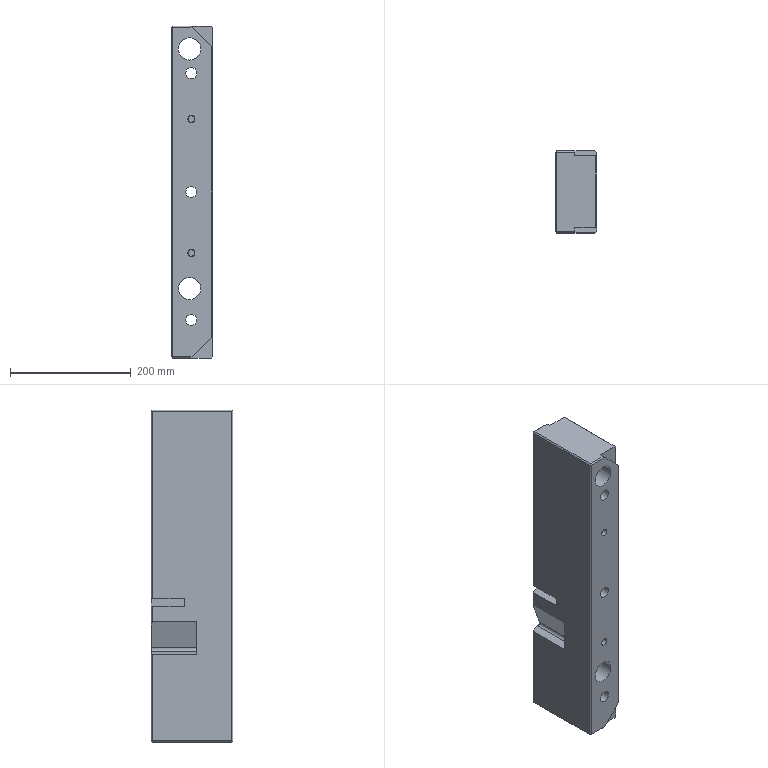Part | STEP file | SPACE-PLATE_id502_x_t | 1 solid | 48 faces | box 68 x 135 x 550 mm | volume 4551876 mm3 | plane 37 | cylinder 9 | cone 2 | commonest cylinder face diameters 18.5 x3 10 x2 12 x2 37 x2
STEP:
#1=CARTESIAN_POINT('',(165.,-234.5,115.75));
#2=VERTEX_POINT('',#1);
#3=CARTESIAN_POINT('',(165.,-234.5,121.));
#4=DIRECTION('',(0.,-1.,0.));
#5=DIRECTION('',(0.,0.,-1.));
#6=AXIS2_PLACEMENT_3D('',#3,#4,#5);
#7=CIRCLE('',#6,5.25);
#8=EDGE_CURVE('',#2,#2,#7,.T.);
#9=ORIENTED_EDGE('',*,*,#8,.T.);
#10=EDGE_LOOP('',(#9));
#11=FACE_OUTER_BOUND('',#10,.T.);
#12=CARTESIAN_POINT('',(165.,-234.5,121.));
#13=DIRECTION('',(0.,1.,0.));
#14=DIRECTION('',(0.,0.,1.));
#15=AXIS2_PLACEMENT_3D('',#12,#13,#14);
#16=PLANE('',#15);
#17=ADVANCED_FACE('',(#11),#16,.F.);
#18=CARTESIAN_POINT('',(165.,-234.5,-106.25));
#19=VERTEX_POINT('',#18);
#20=CARTESIAN_POINT('',(165.,-234.5,-101.));
#21=DIRECTION('',(0.,-1.,0.));
#22=DIRECTION('',(0.,0.,-1.));
#23=AXIS2_PLACEMENT_3D('',#20,#21,#22);
#24=CIRCLE('',#23,5.25);
#25=EDGE_CURVE('',#19,#19,#24,.T.);
#26=ORIENTED_EDGE('',*,*,#25,.T.);
#27=EDGE_LOOP('',(#26));
#28=FACE_OUTER_BOUND('',#27,.T.);
#29=CARTESIAN_POINT('',(165.,-234.5,-101.));
#30=DIRECTION('',(0.,-1.,0.));
#31=DIRECTION('',(0.,0.,-1.));
#32=AXIS2_PLACEMENT_3D('',#29,#30,#31);
#33=PLANE('',#32);
#34=ADVANCED_FACE('',(#28),#33,.T.);
#35=CARTESIAN_POINT('',(165.,-235.25,127.));
#36=VERTEX_POINT('',#35);
#37=CARTESIAN_POINT('',(165.,-235.25,121.));
#38=DIRECTION('',(0.,-1.,0.));
#39=DIRECTION('',(0.,0.,1.));
#40=AXIS2_PLACEMENT_3D('',#37,#38,#39);
#41=CIRCLE('',#40,6.);
#42=EDGE_CURVE('',#36,#36,#41,.T.);
#43=ORIENTED_EDGE('',*,*,#42,.T.);
#44=EDGE_LOOP('',(#43));
#45=FACE_BOUND('',#44,.T.);
#46=ORIENTED_EDGE('',*,*,#8,.F.);
#47=EDGE_LOOP('',(#46));
#48=FACE_BOUND('',#47,.T.);
#49=CARTESIAN_POINT('',(165.,-235.25,121.));
#50=DIRECTION('',(0.,-1.,0.));
#51=DIRECTION('',(0.,0.,-1.));
#52=AXIS2_PLACEMENT_3D('',#49,#50,#51);
#53=CONICAL_SURFACE('',#52,6.,45.);
#54=ADVANCED_FACE('',(#45,#48),#53,.F.);
#55=CARTESIAN_POINT('',(165.,-235.25,-107.));
#56=VERTEX_POINT('',#55);
#57=CARTESIAN_POINT('',(165.,-235.25,-101.));
#58=DIRECTION('',(0.,-1.,0.));
#59=DIRECTION('',(0.,0.,-1.));
#60=AXIS2_PLACEMENT_3D('',#57,#58,#59);
#61=CIRCLE('',#60,6.);
#62=EDGE_CURVE('',#56,#56,#61,.T.);
#63=ORIENTED_EDGE('',*,*,#62,.T.);
#64=EDGE_LOOP('',(#63));
#65=FACE_BOUND('',#64,.T.);
#66=ORIENTED_EDGE('',*,*,#25,.F.);
#67=EDGE_LOOP('',(#66));
#68=FACE_BOUND('',#67,.T.);
#69=CARTESIAN_POINT('',(165.,-235.25,-101.));
#70=DIRECTION('',(0.,-1.,0.));
#71=DIRECTION('',(0.,0.,-1.));
#72=AXIS2_PLACEMENT_3D('',#69,#70,#71);
#73=CONICAL_SURFACE('',#72,6.,45.);
#74=ADVANCED_FACE('',(#65,#68),#73,.F.);
#75=CARTESIAN_POINT('',(144.313,-195.5,-125.297));
#76=VERTEX_POINT('',#75);
#77=CARTESIAN_POINT('',(132.,-195.5,-129.657));
#78=VERTEX_POINT('',#77);
#79=CARTESIAN_POINT('',(144.313,-195.5,-125.297));
#80=DIRECTION('',(-0.9426,0.,-0.3338));
#81=VECTOR('',#80,1.);
#82=LINE('',#79,#81);
#83=EDGE_CURVE('',#76,#78,#82,.T.);
#84=ORIENTED_EDGE('',*,*,#83,.T.);
#85=CARTESIAN_POINT('',(132.,-195.5,-75.548));
#86=VERTEX_POINT('',#85);
#87=CARTESIAN_POINT('',(132.,-195.5,275.));
#88=DIRECTION('',(0.,0.,-1.));
#89=VECTOR('',#88,1.);
#90=LINE('',#87,#89);
#91=EDGE_CURVE('',#86,#78,#90,.T.);
#92=ORIENTED_EDGE('',*,*,#91,.F.);
#93=CARTESIAN_POINT('',(147.357,-195.5,-118.915));
#94=VERTEX_POINT('',#93);
#95=CARTESIAN_POINT('',(132.,-195.5,-75.548));
#96=DIRECTION('',(0.3338,0.,-0.9426));
#97=VECTOR('',#96,1.);
#98=LINE('',#95,#97);
#99=EDGE_CURVE('',#86,#94,#98,.T.);
#100=ORIENTED_EDGE('',*,*,#99,.T.);
#101=CARTESIAN_POINT('',(142.644,-195.5,-120.584));
#102=DIRECTION('',(0.,1.,0.));
#103=DIRECTION('',(0.,0.,1.));
#104=AXIS2_PLACEMENT_3D('',#101,#102,#103);
#105=CIRCLE('',#104,5.);
#106=EDGE_CURVE('',#94,#76,#105,.T.);
#107=ORIENTED_EDGE('',*,*,#106,.T.);
#108=EDGE_LOOP('',(#84,#92,#100,#107));
#109=FACE_OUTER_BOUND('',#108,.T.);
#110=CARTESIAN_POINT('',(-225.,-195.5,275.));
#111=DIRECTION('',(0.,1.,0.));
#112=DIRECTION('',(0.,0.,1.));
#113=AXIS2_PLACEMENT_3D('',#110,#111,#112);
#114=PLANE('',#113);
#115=ADVANCED_FACE('',(#109),#114,.T.);
#116=CARTESIAN_POINT('',(173.488,-175.5,-35.932));
#117=VERTEX_POINT('',#116);
#118=CARTESIAN_POINT('',(132.,-175.5,-50.624));
#119=VERTEX_POINT('',#118);
#120=CARTESIAN_POINT('',(173.488,-175.5,-35.932));
#121=DIRECTION('',(-0.9426,0.,-0.3338));
#122=VECTOR('',#121,1.);
#123=LINE('',#120,#122);
#124=EDGE_CURVE('',#117,#119,#123,.T.);
#125=ORIENTED_EDGE('',*,*,#124,.T.);
#126=CARTESIAN_POINT('',(132.,-175.5,-36.833));
#127=VERTEX_POINT('',#126);
#128=CARTESIAN_POINT('',(132.,-175.5,275.));
#129=DIRECTION('',(0.,0.,-1.));
#130=VECTOR('',#129,1.);
#131=LINE('',#128,#130);
#132=EDGE_CURVE('',#127,#119,#131,.T.);
#133=ORIENTED_EDGE('',*,*,#132,.F.);
#134=CARTESIAN_POINT('',(173.862,-175.5,-22.009));
#135=VERTEX_POINT('',#134);
#136=CARTESIAN_POINT('',(132.,-175.5,-36.833));
#137=DIRECTION('',(0.9426,0.,0.3338));
#138=VECTOR('',#137,1.);
#139=LINE('',#136,#138);
#140=EDGE_CURVE('',#127,#135,#139,.T.);
#141=ORIENTED_EDGE('',*,*,#140,.T.);
#142=CARTESIAN_POINT('',(176.532,-175.5,-29.55));
#143=VERTEX_POINT('',#142);
#144=CARTESIAN_POINT('',(173.862,-175.5,-22.009));
#145=DIRECTION('',(0.3338,0.,-0.9426));
#146=VECTOR('',#145,1.);
#147=LINE('',#144,#146);
#148=EDGE_CURVE('',#135,#143,#147,.T.);
#149=ORIENTED_EDGE('',*,*,#148,.T.);
#150=CARTESIAN_POINT('',(171.819,-175.5,-31.219));
#151=DIRECTION('',(0.,1.,0.));
#152=DIRECTION('',(0.,0.,1.));
#153=AXIS2_PLACEMENT_3D('',#150,#151,#152);
#154=CIRCLE('',#153,5.);
#155=EDGE_CURVE('',#143,#117,#154,.T.);
#156=ORIENTED_EDGE('',*,*,#155,.T.);
#157=EDGE_LOOP('',(#125,#133,#141,#149,#156));
#158=FACE_OUTER_BOUND('',#157,.T.);
#159=CARTESIAN_POINT('',(-225.,-175.5,275.));
#160=DIRECTION('',(0.,1.,0.));
#161=DIRECTION('',(0.,0.,1.));
#162=AXIS2_PLACEMENT_3D('',#159,#160,#161);
#163=PLANE('',#162);
#164=ADVANCED_FACE('',(#158),#163,.T.);
#165=CARTESIAN_POINT('',(132.,-122.5,-36.833));
#166=VERTEX_POINT('',#165);
#167=CARTESIAN_POINT('',(132.,-120.5,-36.833));
#168=DIRECTION('',(0.,-1.,0.));
#169=VECTOR('',#168,1.);
#170=LINE('',#167,#169);
#171=EDGE_CURVE('',#166,#127,#170,.T.);
#172=ORIENTED_EDGE('',*,*,#171,.T.);
#173=ORIENTED_EDGE('',*,*,#132,.T.);
#174=CARTESIAN_POINT('',(132.,-122.5,-50.624));
#175=VERTEX_POINT('',#174);
#176=CARTESIAN_POINT('',(132.,-120.5,-50.624));
#177=DIRECTION('',(0.,1.,0.));
#178=VECTOR('',#177,1.);
#179=LINE('',#176,#178);
#180=EDGE_CURVE('',#119,#175,#179,.T.);
#181=ORIENTED_EDGE('',*,*,#180,.T.);
#182=CARTESIAN_POINT('',(132.,-122.5,-75.548));
#183=VERTEX_POINT('',#182);
#184=CARTESIAN_POINT('',(132.,-122.5,275.));
#185=DIRECTION('',(0.,0.,1.));
#186=VECTOR('',#185,1.);
#187=LINE('',#184,#186);
#188=EDGE_CURVE('',#183,#175,#187,.T.);
#189=ORIENTED_EDGE('',*,*,#188,.F.);
#190=CARTESIAN_POINT('',(132.,-120.5,-75.548));
#191=DIRECTION('',(0.,-1.,0.));
#192=VECTOR('',#191,1.);
#193=LINE('',#190,#192);
#194=EDGE_CURVE('',#183,#86,#193,.T.);
#195=ORIENTED_EDGE('',*,*,#194,.T.);
#196=ORIENTED_EDGE('',*,*,#91,.T.);
#197=CARTESIAN_POINT('',(132.,-122.5,-129.657));
#198=VERTEX_POINT('',#197);
#199=CARTESIAN_POINT('',(132.,-120.5,-129.657));
#200=DIRECTION('',(0.,1.,0.));
#201=VECTOR('',#200,1.);
#202=LINE('',#199,#201);
#203=EDGE_CURVE('',#78,#198,#202,.T.);
#204=ORIENTED_EDGE('',*,*,#203,.T.);
#205=CARTESIAN_POINT('',(132.,-122.5,-273.));
#206=VERTEX_POINT('',#205);
#207=CARTESIAN_POINT('',(132.,-122.5,275.));
#208=DIRECTION('',(0.,0.,1.));
#209=VECTOR('',#208,1.);
#210=LINE('',#207,#209);
#211=EDGE_CURVE('',#206,#198,#210,.T.);
#212=ORIENTED_EDGE('',*,*,#211,.F.);
#213=CARTESIAN_POINT('',(132.,-253.5,-273.));
#214=VERTEX_POINT('',#213);
#215=CARTESIAN_POINT('',(132.,-255.5,-273.));
#216=DIRECTION('',(0.,-1.,0.));
#217=VECTOR('',#216,1.);
#218=LINE('',#215,#217);
#219=EDGE_CURVE('',#206,#214,#218,.T.);
#220=ORIENTED_EDGE('',*,*,#219,.T.);
#221=CARTESIAN_POINT('',(132.,-253.5,273.));
#222=VERTEX_POINT('',#221);
#223=CARTESIAN_POINT('',(132.,-253.5,273.));
#224=DIRECTION('',(0.,0.,-1.));
#225=VECTOR('',#224,1.);
#226=LINE('',#223,#225);
#227=EDGE_CURVE('',#222,#214,#226,.T.);
#228=ORIENTED_EDGE('',*,*,#227,.F.);
#229=CARTESIAN_POINT('',(132.,-122.5,273.));
#230=VERTEX_POINT('',#229);
#231=CARTESIAN_POINT('',(132.,-253.5,273.));
#232=DIRECTION('',(0.,-1.,0.));
#233=VECTOR('',#232,1.);
#234=LINE('',#231,#233);
#235=EDGE_CURVE('',#230,#222,#234,.T.);
#236=ORIENTED_EDGE('',*,*,#235,.F.);
#237=CARTESIAN_POINT('',(132.,-122.5,275.));
#238=DIRECTION('',(0.,0.,1.));
#239=VECTOR('',#238,1.);
#240=LINE('',#237,#239);
#241=EDGE_CURVE('',#166,#230,#240,.T.);
#242=ORIENTED_EDGE('',*,*,#241,.F.);
#243=EDGE_LOOP('',(#172,#173,#181,#189,#195,#196,#204,#212,#220,#228,#236,#242));
#244=FACE_OUTER_BOUND('',#243,.T.);
#245=CARTESIAN_POINT('',(132.,-255.5,275.));
#246=DIRECTION('',(-1.,0.,0.));
#247=DIRECTION('',(0.,0.,1.));
#248=AXIS2_PLACEMENT_3D('',#245,#246,#247);
#249=PLANE('',#248);
#250=ADVANCED_FACE('',(#244),#249,.T.);
#251=CARTESIAN_POINT('',(133.,-254.5,274.));
#252=VERTEX_POINT('',#251);
#253=CARTESIAN_POINT('',(132.,-253.5,273.));
#254=DIRECTION('',(0.5774,-0.5774,0.5774));
#255=VECTOR('',#254,1.);
#256=LINE('',#253,#255);
#257=EDGE_CURVE('',#222,#252,#256,.T.);
#258=ORIENTED_EDGE('',*,*,#257,.F.);
#259=ORIENTED_EDGE('',*,*,#227,.T.);
#260=CARTESIAN_POINT('',(133.,-254.5,-274.));
#261=VERTEX_POINT('',#260);
#262=CARTESIAN_POINT('',(132.,-253.5,-273.));
#263=DIRECTION('',(0.5774,-0.5774,-0.5774));
#264=VECTOR('',#263,1.);
#265=LINE('',#262,#264);
#266=EDGE_CURVE('',#214,#261,#265,.T.);
#267=ORIENTED_EDGE('',*,*,#266,.T.);
#268=CARTESIAN_POINT('',(134.,-255.5,-273.));
#269=VERTEX_POINT('',#268);
#270=CARTESIAN_POINT('',(133.,-254.5,-274.));
#271=DIRECTION('',(0.5774,-0.5774,0.5774));
#272=VECTOR('',#271,1.);
#273=LINE('',#270,#272);
#274=EDGE_CURVE('',#261,#269,#273,.T.);
#275=ORIENTED_EDGE('',*,*,#274,.T.);
#276=CARTESIAN_POINT('',(134.,-255.5,273.));
#277=VERTEX_POINT('',#276);
#278=CARTESIAN_POINT('',(134.,-255.5,275.));
#279=DIRECTION('',(0.,0.,-1.));
#280=VECTOR('',#279,1.);
#281=LINE('',#278,#280);
#282=EDGE_CURVE('',#277,#269,#281,.T.);
#283=ORIENTED_EDGE('',*,*,#282,.F.);
#284=CARTESIAN_POINT('',(133.,-254.5,274.));
#285=DIRECTION('',(0.5774,-0.5774,-0.5774));
#286=VECTOR('',#285,1.);
#287=LINE('',#284,#286);
#288=EDGE_CURVE('',#252,#277,#287,.T.);
#289=ORIENTED_EDGE('',*,*,#288,.F.);
#290=EDGE_LOOP('',(#258,#259,#267,#275,#283,#289));
#291=FACE_OUTER_BOUND('',#290,.T.);
#292=CARTESIAN_POINT('',(132.,-253.5,273.));
#293=DIRECTION('',(-0.7071,-0.7071,0.));
#294=DIRECTION('',(0.7071,-0.7071,0.));
#295=AXIS2_PLACEMENT_3D('',#292,#293,#294);
#296=PLANE('',#295);
#297=ADVANCED_FACE('',(#291),#296,.T.);
#298=ORIENTED_EDGE('',*,*,#42,.F.);
#299=EDGE_LOOP('',(#298));
#300=FACE_BOUND('',#299,.T.);
#301=CARTESIAN_POINT('',(165.,-255.5,127.));
#302=VERTEX_POINT('',#301);
#303=CARTESIAN_POINT('',(165.,-255.5,121.));
#304=DIRECTION('',(0.,1.,0.));
#305=DIRECTION('',(0.,0.,1.));
#306=AXIS2_PLACEMENT_3D('',#303,#304,#305);
#307=CIRCLE('',#306,6.);
#308=EDGE_CURVE('',#302,#302,#307,.T.);
#309=ORIENTED_EDGE('',*,*,#308,.F.);
#310=EDGE_LOOP('',(#309));
#311=FACE_BOUND('',#310,.T.);
#312=CARTESIAN_POINT('',(165.,-292.25,121.));
#313=DIRECTION('',(0.,1.,0.));
#314=DIRECTION('',(0.,0.,1.));
#315=AXIS2_PLACEMENT_3D('',#312,#313,#314);
#316=CYLINDRICAL_SURFACE('',#315,6.);
#317=ADVANCED_FACE('',(#300,#311),#316,.F.);
#318=ORIENTED_EDGE('',*,*,#62,.F.);
#319=EDGE_LOOP('',(#318));
#320=FACE_BOUND('',#319,.T.);
#321=CARTESIAN_POINT('',(165.,-255.5,-107.));
#322=VERTEX_POINT('',#321);
#323=CARTESIAN_POINT('',(165.,-255.5,-101.));
#324=DIRECTION('',(0.,1.,0.));
#325=DIRECTION('',(0.,0.,-1.));
#326=AXIS2_PLACEMENT_3D('',#323,#324,#325);
#327=CIRCLE('',#326,6.);
#328=EDGE_CURVE('',#322,#322,#327,.T.);
#329=ORIENTED_EDGE('',*,*,#328,.F.);
#330=EDGE_LOOP('',(#329));
#331=FACE_BOUND('',#330,.T.);
#332=CARTESIAN_POINT('',(165.,-292.25,-101.));
#333=DIRECTION('',(0.,-1.,0.));
#334=DIRECTION('',(0.,0.,-1.));
#335=AXIS2_PLACEMENT_3D('',#332,#333,#334);
#336=CYLINDRICAL_SURFACE('',#335,6.);
#337=ADVANCED_FACE('',(#320,#331),#336,.F.);
#338=ORIENTED_EDGE('',*,*,#266,.F.);
#339=ORIENTED_EDGE('',*,*,#219,.F.);
#340=CARTESIAN_POINT('',(133.,-121.5,-274.));
#341=VERTEX_POINT('',#340);
#342=CARTESIAN_POINT('',(133.,-121.5,-274.));
#343=DIRECTION('',(-0.5774,-0.5774,0.5774));
#344=VECTOR('',#343,1.);
#345=LINE('',#342,#344);
#346=EDGE_CURVE('',#341,#206,#345,.T.);
#347=ORIENTED_EDGE('',*,*,#346,.F.);
#348=CARTESIAN_POINT('',(134.,-122.5,-275.));
#349=VERTEX_POINT('',#348);
#350=CARTESIAN_POINT('',(133.,-121.5,-274.));
#351=DIRECTION('',(0.5774,-0.5774,-0.5774));
#352=VECTOR('',#351,1.);
#353=LINE('',#350,#352);
#354=EDGE_CURVE('',#341,#349,#353,.T.);
#355=ORIENTED_EDGE('',*,*,#354,.T.);
#356=CARTESIAN_POINT('',(134.,-253.5,-275.));
#357=VERTEX_POINT('',#356);
#358=CARTESIAN_POINT('',(134.,-60.,-275.));
#359=DIRECTION('',(0.,1.,0.));
#360=VECTOR('',#359,1.);
#361=LINE('',#358,#360);
#362=EDGE_CURVE('',#357,#349,#361,.T.);
#363=ORIENTED_EDGE('',*,*,#362,.F.);
#364=CARTESIAN_POINT('',(134.,-253.5,-275.));
#365=DIRECTION('',(-0.5774,-0.5774,0.5774));
#366=VECTOR('',#365,1.);
#367=LINE('',#364,#366);
#368=EDGE_CURVE('',#357,#261,#367,.T.);
#369=ORIENTED_EDGE('',*,*,#368,.T.);
#370=EDGE_LOOP('',(#338,#339,#347,#355,#363,#369));
#371=FACE_OUTER_BOUND('',#370,.T.);
#372=CARTESIAN_POINT('',(134.,-255.5,-275.));
#373=DIRECTION('',(0.7071,0.,0.7071));
#374=DIRECTION('',(0.7071,0.,-0.7071));
#375=AXIS2_PLACEMENT_3D('',#372,#373,#374);
#376=PLANE('',#375);
#377=ADVANCED_FACE('',(#371),#376,.F.);
#378=ORIENTED_EDGE('',*,*,#148,.F.);
#379=CARTESIAN_POINT('',(173.862,-120.5,-22.009));
#380=VERTEX_POINT('',#379);
#381=CARTESIAN_POINT('',(173.862,-120.5,-22.009));
#382=DIRECTION('',(0.,1.,0.));
#383=VECTOR('',#382,1.);
#384=LINE('',#381,#383);
#385=EDGE_CURVE('',#135,#380,#384,.T.);
#386=ORIENTED_EDGE('',*,*,#385,.T.);
#387=CARTESIAN_POINT('',(176.532,-120.5,-29.55));
#388=VERTEX_POINT('',#387);
#389=CARTESIAN_POINT('',(176.532,-120.5,-29.55));
#390=DIRECTION('',(-0.3338,0.,0.9426));
#391=VECTOR('',#390,1.);
#392=LINE('',#389,#391);
#393=EDGE_CURVE('',#388,#380,#392,.T.);
#394=ORIENTED_EDGE('',*,*,#393,.F.);
#395=CARTESIAN_POINT('',(176.532,-120.5,-29.55));
#396=DIRECTION('',(0.,-1.,0.));
#397=VECTOR('',#396,1.);
#398=LINE('',#395,#397);
#399=EDGE_CURVE('',#388,#143,#398,.T.);
#400=ORIENTED_EDGE('',*,*,#399,.T.);
#401=EDGE_LOOP('',(#378,#386,#394,#400));
#402=FACE_OUTER_BOUND('',#401,.T.);
#403=CARTESIAN_POINT('',(173.862,-120.5,-22.009));
#404=DIRECTION('',(0.9426,0.,0.3338));
#405=DIRECTION('',(0.3338,0.,-0.9426));
#406=AXIS2_PLACEMENT_3D('',#403,#404,#405);
#407=PLANE('',#406);
#408=ADVANCED_FACE('',(#402),#407,.F.);
#409=CARTESIAN_POINT('',(134.,-120.5,-36.124));
#410=VERTEX_POINT('',#409);
#411=CARTESIAN_POINT('',(173.862,-120.5,-22.009));
#412=DIRECTION('',(-0.9426,0.,-0.3338));
#413=VECTOR('',#412,1.);
#414=LINE('',#411,#413);
#415=EDGE_CURVE('',#380,#410,#414,.T.);
#416=ORIENTED_EDGE('',*,*,#415,.F.);
#417=ORIENTED_EDGE('',*,*,#385,.F.);
#418=ORIENTED_EDGE('',*,*,#140,.F.);
#419=ORIENTED_EDGE('',*,*,#171,.F.);
#420=CARTESIAN_POINT('',(134.,-120.5,-36.124));
#421=DIRECTION('',(-0.6859,-0.6859,-0.2429));
#422=VECTOR('',#421,1.);
#423=LINE('',#420,#422);
#424=EDGE_CURVE('',#410,#166,#423,.T.);
#425=ORIENTED_EDGE('',*,*,#424,.F.);
#426=EDGE_LOOP('',(#416,#417,#418,#419,#425));
#427=FACE_OUTER_BOUND('',#426,.T.);
#428=CARTESIAN_POINT('',(132.,-120.5,-36.833));
#429=DIRECTION('',(-0.3338,0.,0.9426));
#430=DIRECTION('',(0.9426,0.,0.3338));
#431=AXIS2_PLACEMENT_3D('',#428,#429,#430);
#432=PLANE('',#431);
#433=ADVANCED_FACE('',(#427),#432,.F.);
#434=CARTESIAN_POINT('',(134.,-120.5,273.));
#435=VERTEX_POINT('',#434);
#436=CARTESIAN_POINT('',(134.,-120.5,275.));
#437=DIRECTION('',(0.,0.,1.));
#438=VECTOR('',#437,1.);
#439=LINE('',#436,#438);
#440=EDGE_CURVE('',#410,#435,#439,.T.);
#441=ORIENTED_EDGE('',*,*,#440,.F.);
#442=ORIENTED_EDGE('',*,*,#424,.T.);
#443=ORIENTED_EDGE('',*,*,#241,.T.);
#444=CARTESIAN_POINT('',(133.,-121.5,274.));
#445=VERTEX_POINT('',#444);
#446=CARTESIAN_POINT('',(133.,-121.5,274.));
#447=DIRECTION('',(-0.5774,-0.5774,-0.5774));
#448=VECTOR('',#447,1.);
#449=LINE('',#446,#448);
#450=EDGE_CURVE('',#445,#230,#449,.T.);
#451=ORIENTED_EDGE('',*,*,#450,.F.);
#452=CARTESIAN_POINT('',(134.,-120.5,273.));
#453=DIRECTION('',(-0.5774,-0.5774,0.5774));
#454=VECTOR('',#453,1.);
#455=LINE('',#452,#454);
#456=EDGE_CURVE('',#435,#445,#455,.T.);
#457=ORIENTED_EDGE('',*,*,#456,.F.);
#458=EDGE_LOOP('',(#441,#442,#443,#451,#457));
#459=FACE_OUTER_BOUND('',#458,.T.);
#460=CARTESIAN_POINT('',(134.,-120.5,275.));
#461=DIRECTION('',(-0.7071,0.7071,0.));
#462=DIRECTION('',(-0.7071,-0.7071,0.));
#463=AXIS2_PLACEMENT_3D('',#460,#461,#462);
#464=PLANE('',#463);
#465=ADVANCED_FACE('',(#459),#464,.T.);
#466=ORIENTED_EDGE('',*,*,#211,.T.);
#467=CARTESIAN_POINT('',(134.,-120.5,-128.949));
#468=VERTEX_POINT('',#467);
#469=CARTESIAN_POINT('',(132.,-122.5,-129.657));
#470=DIRECTION('',(0.6859,0.6859,0.2429));
#471=VECTOR('',#470,1.);
#472=LINE('',#469,#471);
#473=EDGE_CURVE('',#198,#468,#472,.T.);
#474=ORIENTED_EDGE('',*,*,#473,.T.);
#475=CARTESIAN_POINT('',(134.,-120.5,-273.));
#476=VERTEX_POINT('',#475);
#477=CARTESIAN_POINT('',(134.,-120.5,275.));
#478=DIRECTION('',(0.,0.,1.));
#479=VECTOR('',#478,1.);
#480=LINE('',#477,#479);
#481=EDGE_CURVE('',#476,#468,#480,.T.);
#482=ORIENTED_EDGE('',*,*,#481,.F.);
#483=CARTESIAN_POINT('',(134.,-120.5,-273.));
#484=DIRECTION('',(-0.5774,-0.5774,-0.5774));
#485=VECTOR('',#484,1.);
#486=LINE('',#483,#485);
#487=EDGE_CURVE('',#476,#341,#486,.T.);
#488=ORIENTED_EDGE('',*,*,#487,.T.);
#489=ORIENTED_EDGE('',*,*,#346,.T.);
#490=EDGE_LOOP('',(#466,#474,#482,#488,#489));
#491=FACE_OUTER_BOUND('',#490,.T.);
#492=CARTESIAN_POINT('',(134.,-120.5,275.));
#493=DIRECTION('',(-0.7071,0.7071,0.));
#494=DIRECTION('',(-0.7071,-0.7071,0.));
#495=AXIS2_PLACEMENT_3D('',#492,#493,#494);
#496=PLANE('',#495);
#497=ADVANCED_FACE('',(#491),#496,.T.);
#498=CARTESIAN_POINT('',(144.313,-120.5,-125.297));
#499=VERTEX_POINT('',#498);
#500=CARTESIAN_POINT('',(144.313,-120.5,-125.297));
#501=DIRECTION('',(0.,1.,0.));
#502=VECTOR('',#501,1.);
#503=LINE('',#500,#502);
#504=EDGE_CURVE('',#76,#499,#503,.T.);
#505=ORIENTED_EDGE('',*,*,#504,.T.);
#506=CARTESIAN_POINT('',(134.,-120.5,-128.949));
#507=DIRECTION('',(0.9426,0.,0.3338));
#508=VECTOR('',#507,1.);
#509=LINE('',#506,#508);
#510=EDGE_CURVE('',#468,#499,#509,.T.);
#511=ORIENTED_EDGE('',*,*,#510,.F.);
#512=ORIENTED_EDGE('',*,*,#473,.F.);
#513=ORIENTED_EDGE('',*,*,#203,.F.);
#514=ORIENTED_EDGE('',*,*,#83,.F.);
#515=EDGE_LOOP('',(#505,#511,#512,#513,#514));
#516=FACE_OUTER_BOUND('',#515,.T.);
#517=CARTESIAN_POINT('',(144.313,-120.5,-125.297));
#518=DIRECTION('',(0.3338,0.,-0.9426));
#519=DIRECTION('',(-0.9426,0.,-0.3338));
#520=AXIS2_PLACEMENT_3D('',#517,#518,#519);
#521=PLANE('',#520);
#522=ADVANCED_FACE('',(#516),#521,.F.);
#523=ORIENTED_EDGE('',*,*,#106,.F.);
#524=CARTESIAN_POINT('',(147.357,-120.5,-118.915));
#525=VERTEX_POINT('',#524);
#526=CARTESIAN_POINT('',(147.357,-120.5,-118.915));
#527=DIRECTION('',(0.,1.,0.));
#528=VECTOR('',#527,1.);
#529=LINE('',#526,#528);
#530=EDGE_CURVE('',#94,#525,#529,.T.);
#531=ORIENTED_EDGE('',*,*,#530,.T.);
#532=CARTESIAN_POINT('',(142.644,-120.5,-120.584));
#533=DIRECTION('',(0.,-1.,0.));
#534=DIRECTION('',(0.,0.,1.));
#535=AXIS2_PLACEMENT_3D('',#532,#533,#534);
#536=CIRCLE('',#535,5.);
#537=EDGE_CURVE('',#499,#525,#536,.T.);
#538=ORIENTED_EDGE('',*,*,#537,.F.);
#539=ORIENTED_EDGE('',*,*,#504,.F.);
#540=EDGE_LOOP('',(#523,#531,#538,#539));
#541=FACE_OUTER_BOUND('',#540,.T.);
#542=CARTESIAN_POINT('',(142.644,-120.5,-120.584));
#543=DIRECTION('',(0.,1.,0.));
#544=DIRECTION('',(0.,0.,1.));
#545=AXIS2_PLACEMENT_3D('',#542,#543,#544);
#546=CYLINDRICAL_SURFACE('',#545,5.);
#547=ADVANCED_FACE('',(#541),#546,.F.);
#548=CARTESIAN_POINT('',(134.,-120.5,-81.196));
#549=VERTEX_POINT('',#548);
#550=CARTESIAN_POINT('',(147.357,-120.5,-118.915));
#551=DIRECTION('',(-0.3338,0.,0.9426));
#552=VECTOR('',#551,1.);
#553=LINE('',#550,#552);
#554=EDGE_CURVE('',#525,#549,#553,.T.);
#555=ORIENTED_EDGE('',*,*,#554,.F.);
#556=ORIENTED_EDGE('',*,*,#530,.F.);
#557=ORIENTED_EDGE('',*,*,#99,.F.);
#558=ORIENTED_EDGE('',*,*,#194,.F.);
#559=CARTESIAN_POINT('',(134.,-120.5,-81.196));
#560=DIRECTION('',(-0.3166,-0.3166,0.8941));
#561=VECTOR('',#560,1.);
#562=LINE('',#559,#561);
#563=EDGE_CURVE('',#549,#183,#562,.T.);
#564=ORIENTED_EDGE('',*,*,#563,.F.);
#565=EDGE_LOOP('',(#555,#556,#557,#558,#564));
#566=FACE_OUTER_BOUND('',#565,.T.);
#567=CARTESIAN_POINT('',(132.,-120.5,-75.548));
#568=DIRECTION('',(0.9426,0.,0.3338));
#569=DIRECTION('',(0.3338,0.,-0.9426));
#570=AXIS2_PLACEMENT_3D('',#567,#568,#569);
#571=PLANE('',#570);
#572=ADVANCED_FACE('',(#566),#571,.F.);
#573=ORIENTED_EDGE('',*,*,#188,.T.);
#574=CARTESIAN_POINT('',(134.,-120.5,-49.915));
#575=VERTEX_POINT('',#574);
#576=CARTESIAN_POINT('',(132.,-122.5,-50.624));
#577=DIRECTION('',(0.6859,0.6859,0.2429));
#578=VECTOR('',#577,1.);
#579=LINE('',#576,#578);
#580=EDGE_CURVE('',#175,#575,#579,.T.);
#581=ORIENTED_EDGE('',*,*,#580,.T.);
#582=CARTESIAN_POINT('',(134.,-120.5,275.));
#583=DIRECTION('',(0.,0.,1.));
#584=VECTOR('',#583,1.);
#585=LINE('',#582,#584);
#586=EDGE_CURVE('',#549,#575,#585,.T.);
#587=ORIENTED_EDGE('',*,*,#586,.F.);
#588=ORIENTED_EDGE('',*,*,#563,.T.);
#589=EDGE_LOOP('',(#573,#581,#587,#588));
#590=FACE_OUTER_BOUND('',#589,.T.);
#591=CARTESIAN_POINT('',(134.,-120.5,275.));
#592=DIRECTION('',(-0.7071,0.7071,0.));
#593=DIRECTION('',(-0.7071,-0.7071,0.));
#594=AXIS2_PLACEMENT_3D('',#591,#592,#593);
#595=PLANE('',#594);
#596=ADVANCED_FACE('',(#590),#595,.T.);
#597=CARTESIAN_POINT('',(173.488,-120.5,-35.932));
#598=VERTEX_POINT('',#597);
#599=CARTESIAN_POINT('',(173.488,-120.5,-35.932));
#600=DIRECTION('',(0.,1.,0.));
#601=VECTOR('',#600,1.);
#602=LINE('',#599,#601);
#603=EDGE_CURVE('',#117,#598,#602,.T.);
#604=ORIENTED_EDGE('',*,*,#603,.T.);
#605=CARTESIAN_POINT('',(134.,-120.5,-49.915));
#606=DIRECTION('',(0.9426,0.,0.3338));
#607=VECTOR('',#606,1.);
#608=LINE('',#605,#607);
#609=EDGE_CURVE('',#575,#598,#608,.T.);
#610=ORIENTED_EDGE('',*,*,#609,.F.);
#611=ORIENTED_EDGE('',*,*,#580,.F.);
#612=ORIENTED_EDGE('',*,*,#180,.F.);
#613=ORIENTED_EDGE('',*,*,#124,.F.);
#614=EDGE_LOOP('',(#604,#610,#611,#612,#613));
#615=FACE_OUTER_BOUND('',#614,.T.);
#616=CARTESIAN_POINT('',(173.488,-120.5,-35.932));
#617=DIRECTION('',(0.3338,0.,-0.9426));
#618=DIRECTION('',(-0.9426,0.,-0.3338));
#619=AXIS2_PLACEMENT_3D('',#616,#617,#618);
#620=PLANE('',#619);
#621=ADVANCED_FACE('',(#615),#620,.F.);
#622=ORIENTED_EDGE('',*,*,#155,.F.);
#623=ORIENTED_EDGE('',*,*,#399,.F.);
#624=CARTESIAN_POINT('',(171.819,-120.5,-31.219));
#625=DIRECTION('',(0.,-1.,0.));
#626=DIRECTION('',(0.,0.,1.));
#627=AXIS2_PLACEMENT_3D('',#624,#625,#626);
#628=CIRCLE('',#627,5.);
#629=EDGE_CURVE('',#598,#388,#628,.T.);
#630=ORIENTED_EDGE('',*,*,#629,.F.);
#631=ORIENTED_EDGE('',*,*,#603,.F.);
#632=EDGE_LOOP('',(#622,#623,#630,#631));
#633=FACE_OUTER_BOUND('',#632,.T.);
#634=CARTESIAN_POINT('',(171.819,-120.5,-31.219));
#635=DIRECTION('',(0.,1.,0.));
#636=DIRECTION('',(0.,0.,1.));
#637=AXIS2_PLACEMENT_3D('',#634,#635,#636);
#638=CYLINDRICAL_SURFACE('',#637,5.);
#639=ADVANCED_FACE('',(#633),#638,.F.);
#640=CARTESIAN_POINT('',(165.,-120.5,-202.75));
#641=VERTEX_POINT('',#640);
#642=CARTESIAN_POINT('',(165.,-120.5,-212.));
#643=DIRECTION('',(0.,-1.,0.));
#644=DIRECTION('',(0.,0.,1.));
#645=AXIS2_PLACEMENT_3D('',#642,#643,#644);
#646=CIRCLE('',#645,9.25);
#647=EDGE_CURVE('',#641,#641,#646,.T.);
#648=ORIENTED_EDGE('',*,*,#647,.F.);
#649=EDGE_LOOP('',(#648));
#650=FACE_BOUND('',#649,.T.);
#651=CARTESIAN_POINT('',(165.,-255.5,-202.75));
#652=VERTEX_POINT('',#651);
#653=CARTESIAN_POINT('',(165.,-255.5,-212.));
#654=DIRECTION('',(0.,1.,0.));
#655=DIRECTION('',(0.,0.,1.));
#656=AXIS2_PLACEMENT_3D('',#653,#654,#655);
#657=CIRCLE('',#656,9.25);
#658=EDGE_CURVE('',#652,#652,#657,.T.);
#659=ORIENTED_EDGE('',*,*,#658,.F.);
#660=EDGE_LOOP('',(#659));
#661=FACE_BOUND('',#660,.T.);
#662=CARTESIAN_POINT('',(165.,-120.5,-212.));
#663=DIRECTION('',(0.,1.,0.));
#664=DIRECTION('',(0.,0.,1.));
#665=AXIS2_PLACEMENT_3D('',#662,#663,#664);
#666=CYLINDRICAL_SURFACE('',#665,9.25);
#667=ADVANCED_FACE('',(#650,#661),#666,.F.);
#668=CARTESIAN_POINT('',(165.,-120.5,206.25));
#669=VERTEX_POINT('',#668);
#670=CARTESIAN_POINT('',(165.,-120.5,197.));
#671=DIRECTION('',(0.,-1.,0.));
#672=DIRECTION('',(0.,0.,1.));
#673=AXIS2_PLACEMENT_3D('',#670,#671,#672);
#674=CIRCLE('',#673,9.25);
#675=EDGE_CURVE('',#669,#669,#674,.T.);
#676=ORIENTED_EDGE('',*,*,#675,.F.);
#677=EDGE_LOOP('',(#676));
#678=FACE_BOUND('',#677,.T.);
#679=CARTESIAN_POINT('',(165.,-255.5,206.25));
#680=VERTEX_POINT('',#679);
#681=CARTESIAN_POINT('',(165.,-255.5,197.));
#682=DIRECTION('',(0.,1.,0.));
#683=DIRECTION('',(0.,0.,1.));
#684=AXIS2_PLACEMENT_3D('',#681,#682,#683);
#685=CIRCLE('',#684,9.25);
#686=EDGE_CURVE('',#680,#680,#685,.T.);
#687=ORIENTED_EDGE('',*,*,#686,.F.);
#688=EDGE_LOOP('',(#687));
#689=FACE_BOUND('',#688,.T.);
#690=CARTESIAN_POINT('',(165.,-120.5,197.));
#691=DIRECTION('',(0.,1.,0.));
#692=DIRECTION('',(0.,0.,1.));
#693=AXIS2_PLACEMENT_3D('',#690,#691,#692);
#694=CYLINDRICAL_SURFACE('',#693,9.25);
#695=ADVANCED_FACE('',(#678,#689),#694,.F.);
#696=CARTESIAN_POINT('',(165.,-120.5,9.25));
#697=VERTEX_POINT('',#696);
#698=CARTESIAN_POINT('',(165.,-120.5,0.));
#699=DIRECTION('',(0.,-1.,0.));
#700=DIRECTION('',(0.,0.,1.));
#701=AXIS2_PLACEMENT_3D('',#698,#699,#700);
#702=CIRCLE('',#701,9.25);
#703=EDGE_CURVE('',#697,#697,#702,.T.);
#704=ORIENTED_EDGE('',*,*,#703,.F.);
#705=EDGE_LOOP('',(#704));
#706=FACE_BOUND('',#705,.T.);
#707=CARTESIAN_POINT('',(165.,-255.5,9.25));
#708=VERTEX_POINT('',#707);
#709=CARTESIAN_POINT('',(165.,-255.5,0.));
#710=DIRECTION('',(0.,1.,0.));
#711=DIRECTION('',(0.,0.,1.));
#712=AXIS2_PLACEMENT_3D('',#709,#710,#711);
#713=CIRCLE('',#712,9.25);
#714=EDGE_CURVE('',#708,#708,#713,.T.);
#715=ORIENTED_EDGE('',*,*,#714,.F.);
#716=EDGE_LOOP('',(#715));
#717=FACE_BOUND('',#716,.T.);
#718=CARTESIAN_POINT('',(165.,-120.5,0.));
#719=DIRECTION('',(0.,1.,0.));
#720=DIRECTION('',(0.,0.,1.));
#721=AXIS2_PLACEMENT_3D('',#718,#719,#720);
#722=CYLINDRICAL_SURFACE('',#721,9.25);
#723=ADVANCED_FACE('',(#706,#717),#722,.F.);
#724=CARTESIAN_POINT('',(162.,-120.5,-141.5));
#725=VERTEX_POINT('',#724);
#726=CARTESIAN_POINT('',(162.,-120.5,-160.));
#727=DIRECTION('',(0.,-1.,0.));
#728=DIRECTION('',(0.,0.,1.));
#729=AXIS2_PLACEMENT_3D('',#726,#727,#728);
#730=CIRCLE('',#729,18.5);
#731=EDGE_CURVE('',#725,#725,#730,.T.);
#732=ORIENTED_EDGE('',*,*,#731,.F.);
#733=EDGE_LOOP('',(#732));
#734=FACE_BOUND('',#733,.T.);
#735=CARTESIAN_POINT('',(162.,-255.5,-141.5));
#736=VERTEX_POINT('',#735);
#737=CARTESIAN_POINT('',(162.,-255.5,-160.));
#738=DIRECTION('',(0.,1.,0.));
#739=DIRECTION('',(0.,0.,1.));
#740=AXIS2_PLACEMENT_3D('',#737,#738,#739);
#741=CIRCLE('',#740,18.5);
#742=EDGE_CURVE('',#736,#736,#741,.T.);
#743=ORIENTED_EDGE('',*,*,#742,.F.);
#744=EDGE_LOOP('',(#743));
#745=FACE_BOUND('',#744,.T.);
#746=CARTESIAN_POINT('',(162.,-120.5,-160.));
#747=DIRECTION('',(0.,1.,0.));
#748=DIRECTION('',(0.,0.,1.));
#749=AXIS2_PLACEMENT_3D('',#746,#747,#748);
#750=CYLINDRICAL_SURFACE('',#749,18.5);
#751=ADVANCED_FACE('',(#734,#745),#750,.F.);
#752=CARTESIAN_POINT('',(162.,-120.5,255.5));
#753=VERTEX_POINT('',#752);
#754=CARTESIAN_POINT('',(162.,-120.5,237.));
#755=DIRECTION('',(0.,-1.,0.));
#756=DIRECTION('',(0.,0.,1.));
#757=AXIS2_PLACEMENT_3D('',#754,#755,#756);
#758=CIRCLE('',#757,18.5);
#759=EDGE_CURVE('',#753,#753,#758,.T.);
#760=ORIENTED_EDGE('',*,*,#759,.F.);
#761=EDGE_LOOP('',(#760));
#762=FACE_BOUND('',#761,.T.);
#763=CARTESIAN_POINT('',(162.,-255.5,255.5));
#764=VERTEX_POINT('',#763);
#765=CARTESIAN_POINT('',(162.,-255.5,237.));
#766=DIRECTION('',(0.,1.,0.));
#767=DIRECTION('',(0.,0.,1.));
#768=AXIS2_PLACEMENT_3D('',#765,#766,#767);
#769=CIRCLE('',#768,18.5);
#770=EDGE_CURVE('',#764,#764,#769,.T.);
#771=ORIENTED_EDGE('',*,*,#770,.F.);
#772=EDGE_LOOP('',(#771));
#773=FACE_BOUND('',#772,.T.);
#774=CARTESIAN_POINT('',(162.,-120.5,237.));
#775=DIRECTION('',(0.,1.,0.));
#776=DIRECTION('',(0.,0.,1.));
#777=AXIS2_PLACEMENT_3D('',#774,#775,#776);
#778=CYLINDRICAL_SURFACE('',#777,18.5);
#779=ADVANCED_FACE('',(#762,#773),#778,.F.);
#780=CARTESIAN_POINT('',(134.,-253.5,275.));
#781=VERTEX_POINT('',#780);
#782=CARTESIAN_POINT('',(134.,-253.5,275.));
#783=DIRECTION('',(-0.5774,-0.5774,-0.5774));
#784=VECTOR('',#783,1.);
#785=LINE('',#782,#784);
#786=EDGE_CURVE('',#781,#252,#785,.T.);
#787=ORIENTED_EDGE('',*,*,#786,.F.);
#788=CARTESIAN_POINT('',(134.,-122.5,275.));
#789=VERTEX_POINT('',#788);
#790=CARTESIAN_POINT('',(134.,175.5,275.));
#791=DIRECTION('',(0.,1.,0.));
#792=VECTOR('',#791,1.);
#793=LINE('',#790,#792);
#794=EDGE_CURVE('',#781,#789,#793,.T.);
#795=ORIENTED_EDGE('',*,*,#794,.T.);
#796=CARTESIAN_POINT('',(133.,-121.5,274.));
#797=DIRECTION('',(0.5774,-0.5774,0.5774));
#798=VECTOR('',#797,1.);
#799=LINE('',#796,#798);
#800=EDGE_CURVE('',#445,#789,#799,.T.);
#801=ORIENTED_EDGE('',*,*,#800,.F.);
#802=ORIENTED_EDGE('',*,*,#450,.T.);
#803=ORIENTED_EDGE('',*,*,#235,.T.);
#804=ORIENTED_EDGE('',*,*,#257,.T.);
#805=EDGE_LOOP('',(#787,#795,#801,#802,#803,#804));
#806=FACE_OUTER_BOUND('',#805,.T.);
#807=CARTESIAN_POINT('',(134.,-253.5,275.));
#808=DIRECTION('',(-0.7071,0.,0.7071));
#809=DIRECTION('',(0.7071,0.,0.7071));
#810=AXIS2_PLACEMENT_3D('',#807,#808,#809);
#811=PLANE('',#810);
#812=ADVANCED_FACE('',(#806),#811,.T.);
#813=CARTESIAN_POINT('',(166.,-255.5,273.));
#814=VERTEX_POINT('',#813);
#815=CARTESIAN_POINT('',(164.,-253.5,275.));
#816=VERTEX_POINT('',#815);
#817=CARTESIAN_POINT('',(166.,-255.5,273.));
#818=DIRECTION('',(-0.5774,0.5774,0.5774));
#819=VECTOR('',#818,1.);
#820=LINE('',#817,#819);
#821=EDGE_CURVE('',#814,#816,#820,.T.);
#822=ORIENTED_EDGE('',*,*,#821,.T.);
#823=CARTESIAN_POINT('',(-225.,-253.5,275.));
#824=DIRECTION('',(-1.,0.,0.));
#825=VECTOR('',#824,1.);
#826=LINE('',#823,#825);
#827=EDGE_CURVE('',#816,#781,#826,.T.);
#828=ORIENTED_EDGE('',*,*,#827,.T.);
#829=ORIENTED_EDGE('',*,*,#786,.T.);
#830=ORIENTED_EDGE('',*,*,#288,.T.);
#831=CARTESIAN_POINT('',(200.,-255.5,273.));
#832=DIRECTION('',(-1.,0.,0.));
#833=VECTOR('',#832,1.);
#834=LINE('',#831,#833);
#835=EDGE_CURVE('',#814,#277,#834,.T.);
#836=ORIENTED_EDGE('',*,*,#835,.F.);
#837=EDGE_LOOP('',(#822,#828,#829,#830,#836));
#838=FACE_OUTER_BOUND('',#837,.T.);
#839=CARTESIAN_POINT('',(164.,-253.5,275.));
#840=DIRECTION('',(0.,-0.7071,0.7071));
#841=DIRECTION('',(0.,-0.7071,-0.7071));
#842=AXIS2_PLACEMENT_3D('',#839,#840,#841);
#843=PLANE('',#842);
#844=ADVANCED_FACE('',(#838),#843,.T.);
#845=CARTESIAN_POINT('',(166.,-255.5,-273.));
#846=VERTEX_POINT('',#845);
#847=CARTESIAN_POINT('',(200.,-255.5,-273.));
#848=DIRECTION('',(1.,0.,0.));
#849=VECTOR('',#848,1.);
#850=LINE('',#847,#849);
#851=EDGE_CURVE('',#269,#846,#850,.T.);
#852=ORIENTED_EDGE('',*,*,#851,.F.);
#853=ORIENTED_EDGE('',*,*,#274,.F.);
#854=ORIENTED_EDGE('',*,*,#368,.F.);
#855=CARTESIAN_POINT('',(164.,-253.5,-275.));
#856=VERTEX_POINT('',#855);
#857=CARTESIAN_POINT('',(-200.,-253.5,-275.));
#858=DIRECTION('',(-1.,0.,0.));
#859=VECTOR('',#858,1.);
#860=LINE('',#857,#859);
#861=EDGE_CURVE('',#856,#357,#860,.T.);
#862=ORIENTED_EDGE('',*,*,#861,.F.);
#863=CARTESIAN_POINT('',(164.,-253.5,-275.));
#864=DIRECTION('',(0.5774,-0.5774,0.5774));
#865=VECTOR('',#864,1.);
#866=LINE('',#863,#865);
#867=EDGE_CURVE('',#856,#846,#866,.T.);
#868=ORIENTED_EDGE('',*,*,#867,.T.);
#869=EDGE_LOOP('',(#852,#853,#854,#862,#868));
#870=FACE_OUTER_BOUND('',#869,.T.);
#871=CARTESIAN_POINT('',(164.,-253.5,-275.));
#872=DIRECTION('',(0.,0.7071,0.7071));
#873=DIRECTION('',(0.,-0.7071,0.7071));
#874=AXIS2_PLACEMENT_3D('',#871,#872,#873);
#875=PLANE('',#874);
#876=ADVANCED_FACE('',(#870),#875,.F.);
#877=ORIENTED_EDGE('',*,*,#770,.T.);
#878=EDGE_LOOP('',(#877));
#879=FACE_BOUND('',#878,.T.);
#880=ORIENTED_EDGE('',*,*,#742,.T.);
#881=EDGE_LOOP('',(#880));
#882=FACE_BOUND('',#881,.T.);
#883=ORIENTED_EDGE('',*,*,#714,.T.);
#884=EDGE_LOOP('',(#883));
#885=FACE_BOUND('',#884,.T.);
#886=ORIENTED_EDGE('',*,*,#686,.T.);
#887=EDGE_LOOP('',(#886));
#888=FACE_BOUND('',#887,.T.);
#889=ORIENTED_EDGE('',*,*,#658,.T.);
#890=EDGE_LOOP('',(#889));
#891=FACE_BOUND('',#890,.T.);
#892=ORIENTED_EDGE('',*,*,#328,.T.);
#893=EDGE_LOOP('',(#892));
#894=FACE_BOUND('',#893,.T.);
#895=ORIENTED_EDGE('',*,*,#308,.T.);
#896=EDGE_LOOP('',(#895));
#897=FACE_BOUND('',#896,.T.);
#898=CARTESIAN_POINT('',(198.,-255.5,241.));
#899=VERTEX_POINT('',#898);
#900=CARTESIAN_POINT('',(198.,-255.5,-241.));
#901=VERTEX_POINT('',#900);
#902=CARTESIAN_POINT('',(198.,-255.5,241.));
#903=DIRECTION('',(0.,0.,-1.));
#904=VECTOR('',#903,1.);
#905=LINE('',#902,#904);
#906=EDGE_CURVE('',#899,#901,#905,.T.);
#907=ORIENTED_EDGE('',*,*,#906,.F.);
#908=CARTESIAN_POINT('',(164.,-255.5,275.));
#909=DIRECTION('',(-0.7071,0.,0.7071));
#910=VECTOR('',#909,1.);
#911=LINE('',#908,#910);
#912=EDGE_CURVE('',#899,#814,#911,.T.);
#913=ORIENTED_EDGE('',*,*,#912,.T.);
#914=ORIENTED_EDGE('',*,*,#835,.T.);
#915=ORIENTED_EDGE('',*,*,#282,.T.);
#916=ORIENTED_EDGE('',*,*,#851,.T.);
#917=CARTESIAN_POINT('',(200.,-255.5,-239.));
#918=DIRECTION('',(0.7071,0.,0.7071));
#919=VECTOR('',#918,1.);
#920=LINE('',#917,#919);
#921=EDGE_CURVE('',#846,#901,#920,.T.);
#922=ORIENTED_EDGE('',*,*,#921,.T.);
#923=EDGE_LOOP('',(#907,#913,#914,#915,#916,#922));
#924=FACE_BOUND('',#923,.T.);
#925=CARTESIAN_POINT('',(200.,-255.5,275.));
#926=DIRECTION('',(0.,-1.,0.));
#927=DIRECTION('',(0.,0.,-1.));
#928=AXIS2_PLACEMENT_3D('',#925,#926,#927);
#929=PLANE('',#928);
#930=ADVANCED_FACE('',(#879,#882,#885,#888,#891,#894,#897,#924),#929,.T.);
#931=ORIENTED_EDGE('',*,*,#487,.F.);
#932=CARTESIAN_POINT('',(166.,-120.5,-273.));
#933=VERTEX_POINT('',#932);
#934=CARTESIAN_POINT('',(132.,-120.5,-273.));
#935=DIRECTION('',(-1.,0.,0.));
#936=VECTOR('',#935,1.);
#937=LINE('',#934,#936);
#938=EDGE_CURVE('',#933,#476,#937,.T.);
#939=ORIENTED_EDGE('',*,*,#938,.F.);
#940=CARTESIAN_POINT('',(164.,-122.5,-275.));
#941=VERTEX_POINT('',#940);
#942=CARTESIAN_POINT('',(166.,-120.5,-273.));
#943=DIRECTION('',(-0.5774,-0.5774,-0.5774));
#944=VECTOR('',#943,1.);
#945=LINE('',#942,#944);
#946=EDGE_CURVE('',#933,#941,#945,.T.);
#947=ORIENTED_EDGE('',*,*,#946,.T.);
#948=CARTESIAN_POINT('',(-200.,-122.5,-275.));
#949=DIRECTION('',(1.,0.,0.));
#950=VECTOR('',#949,1.);
#951=LINE('',#948,#950);
#952=EDGE_CURVE('',#349,#941,#951,.T.);
#953=ORIENTED_EDGE('',*,*,#952,.F.);
#954=ORIENTED_EDGE('',*,*,#354,.F.);
#955=EDGE_LOOP('',(#931,#939,#947,#953,#954));
#956=FACE_OUTER_BOUND('',#955,.T.);
#957=CARTESIAN_POINT('',(132.,-122.5,-275.));
#958=DIRECTION('',(0.,-0.7071,0.7071));
#959=DIRECTION('',(0.,-0.7071,-0.7071));
#960=AXIS2_PLACEMENT_3D('',#957,#958,#959);
#961=PLANE('',#960);
#962=ADVANCED_FACE('',(#956),#961,.F.);
#963=CARTESIAN_POINT('',(198.,-128.5,-275.));
#964=VERTEX_POINT('',#963);
#965=CARTESIAN_POINT('',(198.,-247.5,-275.));
#966=VERTEX_POINT('',#965);
#967=CARTESIAN_POINT('',(198.,-128.5,-275.));
#968=DIRECTION('',(0.,-1.,0.));
#969=VECTOR('',#968,1.);
#970=LINE('',#967,#969);
#971=EDGE_CURVE('',#964,#966,#970,.T.);
#972=ORIENTED_EDGE('',*,*,#971,.T.);
#973=CARTESIAN_POINT('',(164.,-247.5,-275.));
#974=VERTEX_POINT('',#973);
#975=CARTESIAN_POINT('',(-225.,-247.5,-275.));
#976=DIRECTION('',(1.,0.,0.));
#977=VECTOR('',#976,1.);
#978=LINE('',#975,#977);
#979=EDGE_CURVE('',#974,#966,#978,.T.);
#980=ORIENTED_EDGE('',*,*,#979,.F.);
#981=CARTESIAN_POINT('',(164.,-255.5,-275.));
#982=DIRECTION('',(0.,-1.,0.));
#983=VECTOR('',#982,1.);
#984=LINE('',#981,#983);
#985=EDGE_CURVE('',#974,#856,#984,.T.);
#986=ORIENTED_EDGE('',*,*,#985,.T.);
#987=ORIENTED_EDGE('',*,*,#861,.T.);
#988=ORIENTED_EDGE('',*,*,#362,.T.);
#989=ORIENTED_EDGE('',*,*,#952,.T.);
#990=CARTESIAN_POINT('',(164.,-128.5,-275.));
#991=VERTEX_POINT('',#990);
#992=CARTESIAN_POINT('',(164.,-120.5,-275.));
#993=DIRECTION('',(0.,-1.,0.));
#994=VECTOR('',#993,1.);
#995=LINE('',#992,#994);
#996=EDGE_CURVE('',#941,#991,#995,.T.);
#997=ORIENTED_EDGE('',*,*,#996,.T.);
#998=CARTESIAN_POINT('',(-225.,-128.5,-275.));
#999=DIRECTION('',(-1.,0.,0.));
#1000=VECTOR('',#999,1.);
#1001=LINE('',#998,#1000);
#1002=EDGE_CURVE('',#964,#991,#1001,.T.);
#1003=ORIENTED_EDGE('',*,*,#1002,.F.);
#1004=EDGE_LOOP('',(#972,#980,#986,#987,#988,#989,#997,#1003));
#1005=FACE_OUTER_BOUND('',#1004,.T.);
#1006=CARTESIAN_POINT('',(-200.,-60.,-275.));
#1007=DIRECTION('',(0.,0.,-1.));
#1008=DIRECTION('',(-1.,0.,0.));
#1009=AXIS2_PLACEMENT_3D('',#1006,#1007,#1008);
#1010=PLANE('',#1009);
#1011=ADVANCED_FACE('',(#1005),#1010,.T.);
#1012=ORIENTED_EDGE('',*,*,#800,.T.);
#1013=CARTESIAN_POINT('',(164.,-122.5,275.));
#1014=VERTEX_POINT('',#1013);
#1015=CARTESIAN_POINT('',(-225.,-122.5,275.));
#1016=DIRECTION('',(1.,0.,0.));
#1017=VECTOR('',#1016,1.);
#1018=LINE('',#1015,#1017);
#1019=EDGE_CURVE('',#789,#1014,#1018,.T.);
#1020=ORIENTED_EDGE('',*,*,#1019,.T.);
#1021=CARTESIAN_POINT('',(166.,-120.5,273.));
#1022=VERTEX_POINT('',#1021);
#1023=CARTESIAN_POINT('',(164.,-122.5,275.));
#1024=DIRECTION('',(0.5774,0.5774,-0.5774));
#1025=VECTOR('',#1024,1.);
#1026=LINE('',#1023,#1025);
#1027=EDGE_CURVE('',#1014,#1022,#1026,.T.);
#1028=ORIENTED_EDGE('',*,*,#1027,.T.);
#1029=CARTESIAN_POINT('',(132.,-120.5,273.));
#1030=DIRECTION('',(1.,0.,0.));
#1031=VECTOR('',#1030,1.);
#1032=LINE('',#1029,#1031);
#1033=EDGE_CURVE('',#435,#1022,#1032,.T.);
#1034=ORIENTED_EDGE('',*,*,#1033,.F.);
#1035=ORIENTED_EDGE('',*,*,#456,.T.);
#1036=EDGE_LOOP('',(#1012,#1020,#1028,#1034,#1035));
#1037=FACE_OUTER_BOUND('',#1036,.T.);
#1038=CARTESIAN_POINT('',(134.,-122.5,275.));
#1039=DIRECTION('',(0.,0.7071,0.7071));
#1040=DIRECTION('',(0.,-0.7071,0.7071));
#1041=AXIS2_PLACEMENT_3D('',#1038,#1039,#1040);
#1042=PLANE('',#1041);
#1043=ADVANCED_FACE('',(#1037),#1042,.T.);
#1044=ORIENTED_EDGE('',*,*,#759,.T.);
#1045=EDGE_LOOP('',(#1044));
#1046=FACE_BOUND('',#1045,.T.);
#1047=ORIENTED_EDGE('',*,*,#731,.T.);
#1048=EDGE_LOOP('',(#1047));
#1049=FACE_BOUND('',#1048,.T.);
#1050=ORIENTED_EDGE('',*,*,#703,.T.);
#1051=EDGE_LOOP('',(#1050));
#1052=FACE_BOUND('',#1051,.T.);
#1053=ORIENTED_EDGE('',*,*,#675,.T.);
#1054=EDGE_LOOP('',(#1053));
#1055=FACE_BOUND('',#1054,.T.);
#1056=ORIENTED_EDGE('',*,*,#647,.T.);
#1057=EDGE_LOOP('',(#1056));
#1058=FACE_BOUND('',#1057,.T.);
#1059=ORIENTED_EDGE('',*,*,#609,.T.);
#1060=ORIENTED_EDGE('',*,*,#629,.T.);
#1061=ORIENTED_EDGE('',*,*,#393,.T.);
#1062=ORIENTED_EDGE('',*,*,#415,.T.);
#1063=ORIENTED_EDGE('',*,*,#440,.T.);
#1064=ORIENTED_EDGE('',*,*,#1033,.T.);
#1065=CARTESIAN_POINT('',(198.,-120.5,241.));
#1066=VERTEX_POINT('',#1065);
#1067=CARTESIAN_POINT('',(200.,-120.5,239.));
#1068=DIRECTION('',(0.7071,0.,-0.7071));
#1069=VECTOR('',#1068,1.);
#1070=LINE('',#1067,#1069);
#1071=EDGE_CURVE('',#1022,#1066,#1070,.T.);
#1072=ORIENTED_EDGE('',*,*,#1071,.T.);
#1073=CARTESIAN_POINT('',(198.,-120.5,-241.));
#1074=VERTEX_POINT('',#1073);
#1075=CARTESIAN_POINT('',(198.,-120.5,239.));
#1076=DIRECTION('',(0.,0.,1.));
#1077=VECTOR('',#1076,1.);
#1078=LINE('',#1075,#1077);
#1079=EDGE_CURVE('',#1074,#1066,#1078,.T.);
#1080=ORIENTED_EDGE('',*,*,#1079,.F.);
#1081=CARTESIAN_POINT('',(164.,-120.5,-275.));
#1082=DIRECTION('',(-0.7071,0.,-0.7071));
#1083=VECTOR('',#1082,1.);
#1084=LINE('',#1081,#1083);
#1085=EDGE_CURVE('',#1074,#933,#1084,.T.);
#1086=ORIENTED_EDGE('',*,*,#1085,.T.);
#1087=ORIENTED_EDGE('',*,*,#938,.T.);
#1088=ORIENTED_EDGE('',*,*,#481,.T.);
#1089=ORIENTED_EDGE('',*,*,#510,.T.);
#1090=ORIENTED_EDGE('',*,*,#537,.T.);
#1091=ORIENTED_EDGE('',*,*,#554,.T.);
#1092=ORIENTED_EDGE('',*,*,#586,.T.);
#1093=EDGE_LOOP('',(#1059,#1060,#1061,#1062,#1063,#1064,#1072,#1080,#1086,#1087,#1088,#1089,#1090,#1091,#1092));
#1094=FACE_BOUND('',#1093,.T.);
#1095=CARTESIAN_POINT('',(132.,-120.5,275.));
#1096=DIRECTION('',(0.,1.,0.));
#1097=DIRECTION('',(0.,0.,1.));
#1098=AXIS2_PLACEMENT_3D('',#1095,#1096,#1097);
#1099=PLANE('',#1098);
#1100=ADVANCED_FACE('',(#1046,#1049,#1052,#1055,#1058,#1094),#1099,.T.);
#1101=CARTESIAN_POINT('',(164.,-128.5,275.));
#1102=VERTEX_POINT('',#1101);
#1103=CARTESIAN_POINT('',(198.,-128.5,275.));
#1104=VERTEX_POINT('',#1103);
#1105=CARTESIAN_POINT('',(-225.,-128.5,275.));
#1106=DIRECTION('',(1.,0.,0.));
#1107=VECTOR('',#1106,1.);
#1108=LINE('',#1105,#1107);
#1109=EDGE_CURVE('',#1102,#1104,#1108,.T.);
#1110=ORIENTED_EDGE('',*,*,#1109,.F.);
#1111=CARTESIAN_POINT('',(164.,-120.5,275.));
#1112=DIRECTION('',(0.,1.,0.));
#1113=VECTOR('',#1112,1.);
#1114=LINE('',#1111,#1113);
#1115=EDGE_CURVE('',#1102,#1014,#1114,.T.);
#1116=ORIENTED_EDGE('',*,*,#1115,.T.);
#1117=ORIENTED_EDGE('',*,*,#1019,.F.);
#1118=ORIENTED_EDGE('',*,*,#794,.F.);
#1119=ORIENTED_EDGE('',*,*,#827,.F.);
#1120=CARTESIAN_POINT('',(164.,-247.5,275.));
#1121=VERTEX_POINT('',#1120);
#1122=CARTESIAN_POINT('',(164.,-255.5,275.));
#1123=DIRECTION('',(0.,1.,0.));
#1124=VECTOR('',#1123,1.);
#1125=LINE('',#1122,#1124);
#1126=EDGE_CURVE('',#816,#1121,#1125,.T.);
#1127=ORIENTED_EDGE('',*,*,#1126,.T.);
#1128=CARTESIAN_POINT('',(198.,-247.5,275.));
#1129=VERTEX_POINT('',#1128);
#1130=CARTESIAN_POINT('',(-225.,-247.5,275.));
#1131=DIRECTION('',(-1.,0.,0.));
#1132=VECTOR('',#1131,1.);
#1133=LINE('',#1130,#1132);
#1134=EDGE_CURVE('',#1129,#1121,#1133,.T.);
#1135=ORIENTED_EDGE('',*,*,#1134,.F.);
#1136=CARTESIAN_POINT('',(198.,-128.5,275.));
#1137=DIRECTION('',(0.,-1.,0.));
#1138=VECTOR('',#1137,1.);
#1139=LINE('',#1136,#1138);
#1140=EDGE_CURVE('',#1104,#1129,#1139,.T.);
#1141=ORIENTED_EDGE('',*,*,#1140,.F.);
#1142=EDGE_LOOP('',(#1110,#1116,#1117,#1118,#1119,#1127,#1135,#1141));
#1143=FACE_OUTER_BOUND('',#1142,.T.);
#1144=CARTESIAN_POINT('',(-225.,175.5,275.));
#1145=DIRECTION('',(0.,0.,-1.));
#1146=DIRECTION('',(-1.,0.,0.));
#1147=AXIS2_PLACEMENT_3D('',#1144,#1145,#1146);
#1148=PLANE('',#1147);
#1149=ADVANCED_FACE('',(#1143),#1148,.F.);
#1150=ORIENTED_EDGE('',*,*,#912,.F.);
#1151=CARTESIAN_POINT('',(200.,-253.5,239.));
#1152=VERTEX_POINT('',#1151);
#1153=CARTESIAN_POINT('',(200.,-253.5,239.));
#1154=DIRECTION('',(-0.5774,-0.5774,0.5774));
#1155=VECTOR('',#1154,1.);
#1156=LINE('',#1153,#1155);
#1157=EDGE_CURVE('',#1152,#899,#1156,.T.);
#1158=ORIENTED_EDGE('',*,*,#1157,.F.);
#1159=CARTESIAN_POINT('',(200.,-247.5,239.));
#1160=VERTEX_POINT('',#1159);
#1161=CARTESIAN_POINT('',(200.,-120.5,239.));
#1162=DIRECTION('',(0.,-1.,0.));
#1163=VECTOR('',#1162,1.);
#1164=LINE('',#1161,#1163);
#1165=EDGE_CURVE('',#1160,#1152,#1164,.T.);
#1166=ORIENTED_EDGE('',*,*,#1165,.F.);
#1167=CARTESIAN_POINT('',(164.,-247.5,275.));
#1168=DIRECTION('',(0.7071,0.,-0.7071));
#1169=VECTOR('',#1168,1.);
#1170=LINE('',#1167,#1169);
#1171=EDGE_CURVE('',#1121,#1160,#1170,.T.);
#1172=ORIENTED_EDGE('',*,*,#1171,.F.);
#1173=ORIENTED_EDGE('',*,*,#1126,.F.);
#1174=ORIENTED_EDGE('',*,*,#821,.F.);
#1175=EDGE_LOOP('',(#1150,#1158,#1166,#1172,#1173,#1174));
#1176=FACE_OUTER_BOUND('',#1175,.T.);
#1177=CARTESIAN_POINT('',(164.,-255.5,275.));
#1178=DIRECTION('',(-0.7071,0.,-0.7071));
#1179=DIRECTION('',(-0.7071,0.,0.7071));
#1180=AXIS2_PLACEMENT_3D('',#1177,#1178,#1179);
#1181=PLANE('',#1180);
#1182=ADVANCED_FACE('',(#1176),#1181,.F.);
#1183=ORIENTED_EDGE('',*,*,#1157,.T.);
#1184=ORIENTED_EDGE('',*,*,#906,.T.);
#1185=CARTESIAN_POINT('',(200.,-253.5,-239.));
#1186=VERTEX_POINT('',#1185);
#1187=CARTESIAN_POINT('',(198.,-255.5,-241.));
#1188=DIRECTION('',(0.5774,0.5774,0.5774));
#1189=VECTOR('',#1188,1.);
#1190=LINE('',#1187,#1189);
#1191=EDGE_CURVE('',#901,#1186,#1190,.T.);
#1192=ORIENTED_EDGE('',*,*,#1191,.T.);
#1193=CARTESIAN_POINT('',(200.,-253.5,275.));
#1194=DIRECTION('',(0.,0.,-1.));
#1195=VECTOR('',#1194,1.);
#1196=LINE('',#1193,#1195);
#1197=EDGE_CURVE('',#1152,#1186,#1196,.T.);
#1198=ORIENTED_EDGE('',*,*,#1197,.F.);
#1199=EDGE_LOOP('',(#1183,#1184,#1192,#1198));
#1200=FACE_OUTER_BOUND('',#1199,.T.);
#1201=CARTESIAN_POINT('',(198.,-255.5,241.));
#1202=DIRECTION('',(0.7071,-0.7071,0.));
#1203=DIRECTION('',(0.7071,0.7071,0.));
#1204=AXIS2_PLACEMENT_3D('',#1201,#1202,#1203);
#1205=PLANE('',#1204);
#1206=ADVANCED_FACE('',(#1200),#1205,.T.);
#1207=ORIENTED_EDGE('',*,*,#921,.F.);
#1208=ORIENTED_EDGE('',*,*,#867,.F.);
#1209=ORIENTED_EDGE('',*,*,#985,.F.);
#1210=CARTESIAN_POINT('',(200.,-247.5,-239.));
#1211=VERTEX_POINT('',#1210);
#1212=CARTESIAN_POINT('',(200.,-247.5,-239.));
#1213=DIRECTION('',(-0.7071,0.,-0.7071));
#1214=VECTOR('',#1213,1.);
#1215=LINE('',#1212,#1214);
#1216=EDGE_CURVE('',#1211,#974,#1215,.T.);
#1217=ORIENTED_EDGE('',*,*,#1216,.F.);
#1218=CARTESIAN_POINT('',(200.,-120.5,-239.));
#1219=DIRECTION('',(0.,1.,0.));
#1220=VECTOR('',#1219,1.);
#1221=LINE('',#1218,#1220);
#1222=EDGE_CURVE('',#1186,#1211,#1221,.T.);
#1223=ORIENTED_EDGE('',*,*,#1222,.F.);
#1224=ORIENTED_EDGE('',*,*,#1191,.F.);
#1225=EDGE_LOOP('',(#1207,#1208,#1209,#1217,#1223,#1224));
#1226=FACE_OUTER_BOUND('',#1225,.T.);
#1227=CARTESIAN_POINT('',(200.,-255.5,-239.));
#1228=DIRECTION('',(-0.7071,0.,0.7071));
#1229=DIRECTION('',(0.7071,0.,0.7071));
#1230=AXIS2_PLACEMENT_3D('',#1227,#1228,#1229);
#1231=PLANE('',#1230);
#1232=ADVANCED_FACE('',(#1226),#1231,.F.);
#1233=CARTESIAN_POINT('',(200.,-247.5,-273.));
#1234=VERTEX_POINT('',#1233);
#1235=CARTESIAN_POINT('',(198.,-247.5,-275.));
#1236=DIRECTION('',(0.7071,0.,0.7071));
#1237=VECTOR('',#1236,1.);
#1238=LINE('',#1235,#1237);
#1239=EDGE_CURVE('',#966,#1234,#1238,.T.);
#1240=ORIENTED_EDGE('',*,*,#1239,.T.);
#1241=CARTESIAN_POINT('',(200.,-247.5,275.));
#1242=DIRECTION('',(0.,0.,-1.));
#1243=VECTOR('',#1242,1.);
#1244=LINE('',#1241,#1243);
#1245=EDGE_CURVE('',#1211,#1234,#1244,.T.);
#1246=ORIENTED_EDGE('',*,*,#1245,.F.);
#1247=ORIENTED_EDGE('',*,*,#1216,.T.);
#1248=ORIENTED_EDGE('',*,*,#979,.T.);
#1249=EDGE_LOOP('',(#1240,#1246,#1247,#1248));
#1250=FACE_OUTER_BOUND('',#1249,.T.);
#1251=CARTESIAN_POINT('',(-225.,-247.5,275.));
#1252=DIRECTION('',(0.,-1.,0.));
#1253=DIRECTION('',(0.,0.,-1.));
#1254=AXIS2_PLACEMENT_3D('',#1251,#1252,#1253);
#1255=PLANE('',#1254);
#1256=ADVANCED_FACE('',(#1250),#1255,.T.);
#1257=CARTESIAN_POINT('',(200.,-128.5,-273.));
#1258=VERTEX_POINT('',#1257);
#1259=CARTESIAN_POINT('',(200.,-120.5,-273.));
#1260=DIRECTION('',(0.,1.,0.));
#1261=VECTOR('',#1260,1.);
#1262=LINE('',#1259,#1261);
#1263=EDGE_CURVE('',#1234,#1258,#1262,.T.);
#1264=ORIENTED_EDGE('',*,*,#1263,.F.);
#1265=ORIENTED_EDGE('',*,*,#1239,.F.);
#1266=ORIENTED_EDGE('',*,*,#971,.F.);
#1267=CARTESIAN_POINT('',(200.,-128.5,-273.));
#1268=DIRECTION('',(-0.7071,0.,-0.7071));
#1269=VECTOR('',#1268,1.);
#1270=LINE('',#1267,#1269);
#1271=EDGE_CURVE('',#1258,#964,#1270,.T.);
#1272=ORIENTED_EDGE('',*,*,#1271,.F.);
#1273=EDGE_LOOP('',(#1264,#1265,#1266,#1272));
#1274=FACE_OUTER_BOUND('',#1273,.T.);
#1275=CARTESIAN_POINT('',(198.,-128.5,-275.));
#1276=DIRECTION('',(-0.7071,0.,0.7071));
#1277=DIRECTION('',(0.7071,0.,0.7071));
#1278=AXIS2_PLACEMENT_3D('',#1275,#1276,#1277);
#1279=PLANE('',#1278);
#1280=ADVANCED_FACE('',(#1274),#1279,.F.);
#1281=CARTESIAN_POINT('',(200.,-128.5,-239.));
#1282=VERTEX_POINT('',#1281);
#1283=CARTESIAN_POINT('',(164.,-128.5,-275.));
#1284=DIRECTION('',(0.7071,0.,0.7071));
#1285=VECTOR('',#1284,1.);
#1286=LINE('',#1283,#1285);
#1287=EDGE_CURVE('',#991,#1282,#1286,.T.);
#1288=ORIENTED_EDGE('',*,*,#1287,.T.);
#1289=CARTESIAN_POINT('',(200.,-128.5,275.));
#1290=DIRECTION('',(0.,0.,1.));
#1291=VECTOR('',#1290,1.);
#1292=LINE('',#1289,#1291);
#1293=EDGE_CURVE('',#1258,#1282,#1292,.T.);
#1294=ORIENTED_EDGE('',*,*,#1293,.F.);
#1295=ORIENTED_EDGE('',*,*,#1271,.T.);
#1296=ORIENTED_EDGE('',*,*,#1002,.T.);
#1297=EDGE_LOOP('',(#1288,#1294,#1295,#1296));
#1298=FACE_OUTER_BOUND('',#1297,.T.);
#1299=CARTESIAN_POINT('',(-225.,-128.5,275.));
#1300=DIRECTION('',(0.,1.,0.));
#1301=DIRECTION('',(0.,0.,1.));
#1302=AXIS2_PLACEMENT_3D('',#1299,#1300,#1301);
#1303=PLANE('',#1302);
#1304=ADVANCED_FACE('',(#1298),#1303,.T.);
#1305=ORIENTED_EDGE('',*,*,#996,.F.);
#1306=ORIENTED_EDGE('',*,*,#946,.F.);
#1307=ORIENTED_EDGE('',*,*,#1085,.F.);
#1308=CARTESIAN_POINT('',(200.,-122.5,-239.));
#1309=VERTEX_POINT('',#1308);
#1310=CARTESIAN_POINT('',(200.,-122.5,-239.));
#1311=DIRECTION('',(-0.5774,0.5774,-0.5774));
#1312=VECTOR('',#1311,1.);
#1313=LINE('',#1310,#1312);
#1314=EDGE_CURVE('',#1309,#1074,#1313,.T.);
#1315=ORIENTED_EDGE('',*,*,#1314,.F.);
#1316=CARTESIAN_POINT('',(200.,-120.5,-239.));
#1317=DIRECTION('',(0.,1.,0.));
#1318=VECTOR('',#1317,1.);
#1319=LINE('',#1316,#1318);
#1320=EDGE_CURVE('',#1282,#1309,#1319,.T.);
#1321=ORIENTED_EDGE('',*,*,#1320,.F.);
#1322=ORIENTED_EDGE('',*,*,#1287,.F.);
#1323=EDGE_LOOP('',(#1305,#1306,#1307,#1315,#1321,#1322));
#1324=FACE_OUTER_BOUND('',#1323,.T.);
#1325=CARTESIAN_POINT('',(164.,-120.5,-275.));
#1326=DIRECTION('',(-0.7071,0.,0.7071));
#1327=DIRECTION('',(0.7071,0.,0.7071));
#1328=AXIS2_PLACEMENT_3D('',#1325,#1326,#1327);
#1329=PLANE('',#1328);
#1330=ADVANCED_FACE('',(#1324),#1329,.F.);
#1331=CARTESIAN_POINT('',(200.,-122.5,239.));
#1332=VERTEX_POINT('',#1331);
#1333=CARTESIAN_POINT('',(198.,-120.5,241.));
#1334=DIRECTION('',(0.5774,-0.5774,-0.5774));
#1335=VECTOR('',#1334,1.);
#1336=LINE('',#1333,#1335);
#1337=EDGE_CURVE('',#1066,#1332,#1336,.T.);
#1338=ORIENTED_EDGE('',*,*,#1337,.T.);
#1339=CARTESIAN_POINT('',(200.,-122.5,275.));
#1340=DIRECTION('',(0.,0.,1.));
#1341=VECTOR('',#1340,1.);
#1342=LINE('',#1339,#1341);
#1343=EDGE_CURVE('',#1309,#1332,#1342,.T.);
#1344=ORIENTED_EDGE('',*,*,#1343,.F.);
#1345=ORIENTED_EDGE('',*,*,#1314,.T.);
#1346=ORIENTED_EDGE('',*,*,#1079,.T.);
#1347=EDGE_LOOP('',(#1338,#1344,#1345,#1346));
#1348=FACE_OUTER_BOUND('',#1347,.T.);
#1349=CARTESIAN_POINT('',(200.,-122.5,239.));
#1350=DIRECTION('',(0.7071,0.7071,0.));
#1351=DIRECTION('',(-0.7071,0.7071,0.));
#1352=AXIS2_PLACEMENT_3D('',#1349,#1350,#1351);
#1353=PLANE('',#1352);
#1354=ADVANCED_FACE('',(#1348),#1353,.T.);
#1355=CARTESIAN_POINT('',(200.,-128.5,239.));
#1356=VERTEX_POINT('',#1355);
#1357=CARTESIAN_POINT('',(200.,-120.5,239.));
#1358=DIRECTION('',(0.,-1.,0.));
#1359=VECTOR('',#1358,1.);
#1360=LINE('',#1357,#1359);
#1361=EDGE_CURVE('',#1332,#1356,#1360,.T.);
#1362=ORIENTED_EDGE('',*,*,#1361,.F.);
#1363=ORIENTED_EDGE('',*,*,#1337,.F.);
#1364=ORIENTED_EDGE('',*,*,#1071,.F.);
#1365=ORIENTED_EDGE('',*,*,#1027,.F.);
#1366=ORIENTED_EDGE('',*,*,#1115,.F.);
#1367=CARTESIAN_POINT('',(200.,-128.5,239.));
#1368=DIRECTION('',(-0.7071,0.,0.7071));
#1369=VECTOR('',#1368,1.);
#1370=LINE('',#1367,#1369);
#1371=EDGE_CURVE('',#1356,#1102,#1370,.T.);
#1372=ORIENTED_EDGE('',*,*,#1371,.F.);
#1373=EDGE_LOOP('',(#1362,#1363,#1364,#1365,#1366,#1372));
#1374=FACE_OUTER_BOUND('',#1373,.T.);
#1375=CARTESIAN_POINT('',(200.,-120.5,239.));
#1376=DIRECTION('',(-0.7071,0.,-0.7071));
#1377=DIRECTION('',(-0.7071,0.,0.7071));
#1378=AXIS2_PLACEMENT_3D('',#1375,#1376,#1377);
#1379=PLANE('',#1378);
#1380=ADVANCED_FACE('',(#1374),#1379,.F.);
#1381=ORIENTED_EDGE('',*,*,#1371,.T.);
#1382=ORIENTED_EDGE('',*,*,#1109,.T.);
#1383=CARTESIAN_POINT('',(200.,-128.5,273.));
#1384=VERTEX_POINT('',#1383);
#1385=CARTESIAN_POINT('',(198.,-128.5,275.));
#1386=DIRECTION('',(-0.7071,0.,0.7071));
#1387=VECTOR('',#1386,1.);
#1388=LINE('',#1385,#1387);
#1389=EDGE_CURVE('',#1384,#1104,#1388,.T.);
#1390=ORIENTED_EDGE('',*,*,#1389,.F.);
#1391=CARTESIAN_POINT('',(200.,-128.5,275.));
#1392=DIRECTION('',(0.,0.,1.));
#1393=VECTOR('',#1392,1.);
#1394=LINE('',#1391,#1393);
#1395=EDGE_CURVE('',#1356,#1384,#1394,.T.);
#1396=ORIENTED_EDGE('',*,*,#1395,.F.);
#1397=EDGE_LOOP('',(#1381,#1382,#1390,#1396));
#1398=FACE_OUTER_BOUND('',#1397,.T.);
#1399=CARTESIAN_POINT('',(-225.,-128.5,275.));
#1400=DIRECTION('',(0.,1.,0.));
#1401=DIRECTION('',(0.,0.,1.));
#1402=AXIS2_PLACEMENT_3D('',#1399,#1400,#1401);
#1403=PLANE('',#1402);
#1404=ADVANCED_FACE('',(#1398),#1403,.T.);
#1405=ORIENTED_EDGE('',*,*,#1389,.T.);
#1406=ORIENTED_EDGE('',*,*,#1140,.T.);
#1407=CARTESIAN_POINT('',(200.,-247.5,273.));
#1408=VERTEX_POINT('',#1407);
#1409=CARTESIAN_POINT('',(200.,-247.5,273.));
#1410=DIRECTION('',(-0.7071,0.,0.7071));
#1411=VECTOR('',#1410,1.);
#1412=LINE('',#1409,#1411);
#1413=EDGE_CURVE('',#1408,#1129,#1412,.T.);
#1414=ORIENTED_EDGE('',*,*,#1413,.F.);
#1415=CARTESIAN_POINT('',(200.,-120.5,273.));
#1416=DIRECTION('',(0.,-1.,0.));
#1417=VECTOR('',#1416,1.);
#1418=LINE('',#1415,#1417);
#1419=EDGE_CURVE('',#1384,#1408,#1418,.T.);
#1420=ORIENTED_EDGE('',*,*,#1419,.F.);
#1421=EDGE_LOOP('',(#1405,#1406,#1414,#1420));
#1422=FACE_OUTER_BOUND('',#1421,.T.);
#1423=CARTESIAN_POINT('',(198.,-128.5,275.));
#1424=DIRECTION('',(0.7071,0.,0.7071));
#1425=DIRECTION('',(0.7071,0.,-0.7071));
#1426=AXIS2_PLACEMENT_3D('',#1423,#1424,#1425);
#1427=PLANE('',#1426);
#1428=ADVANCED_FACE('',(#1422),#1427,.T.);
#1429=ORIENTED_EDGE('',*,*,#1413,.T.);
#1430=ORIENTED_EDGE('',*,*,#1134,.T.);
#1431=ORIENTED_EDGE('',*,*,#1171,.T.);
#1432=CARTESIAN_POINT('',(200.,-247.5,275.));
#1433=DIRECTION('',(0.,0.,-1.));
#1434=VECTOR('',#1433,1.);
#1435=LINE('',#1432,#1434);
#1436=EDGE_CURVE('',#1408,#1160,#1435,.T.);
#1437=ORIENTED_EDGE('',*,*,#1436,.F.);
#1438=EDGE_LOOP('',(#1429,#1430,#1431,#1437));
#1439=FACE_OUTER_BOUND('',#1438,.T.);
#1440=CARTESIAN_POINT('',(-225.,-247.5,275.));
#1441=DIRECTION('',(0.,-1.,0.));
#1442=DIRECTION('',(0.,0.,-1.));
#1443=AXIS2_PLACEMENT_3D('',#1440,#1441,#1442);
#1444=PLANE('',#1443);
#1445=ADVANCED_FACE('',(#1439),#1444,.T.);
#1446=ORIENTED_EDGE('',*,*,#1419,.T.);
#1447=ORIENTED_EDGE('',*,*,#1436,.T.);
#1448=ORIENTED_EDGE('',*,*,#1165,.T.);
#1449=ORIENTED_EDGE('',*,*,#1197,.T.);
#1450=ORIENTED_EDGE('',*,*,#1222,.T.);
#1451=ORIENTED_EDGE('',*,*,#1245,.T.);
#1452=ORIENTED_EDGE('',*,*,#1263,.T.);
#1453=ORIENTED_EDGE('',*,*,#1293,.T.);
#1454=ORIENTED_EDGE('',*,*,#1320,.T.);
#1455=ORIENTED_EDGE('',*,*,#1343,.T.);
#1456=ORIENTED_EDGE('',*,*,#1361,.T.);
#1457=ORIENTED_EDGE('',*,*,#1395,.T.);
#1458=EDGE_LOOP('',(#1446,#1447,#1448,#1449,#1450,#1451,#1452,#1453,#1454,#1455,#1456,#1457));
#1459=FACE_OUTER_BOUND('',#1458,.T.);
#1460=CARTESIAN_POINT('',(200.,-120.5,275.));
#1461=DIRECTION('',(1.,0.,0.));
#1462=DIRECTION('',(0.,0.,-1.));
#1463=AXIS2_PLACEMENT_3D('',#1460,#1461,#1462);
#1464=PLANE('',#1463);
#1465=ADVANCED_FACE('',(#1459),#1464,.T.);
#1466=CLOSED_SHELL('',(#17,#34,#54,#74,#115,#164,#250,#297,#317,#337,#377,#408,#433,#465,#497,#522,#547,#572,#596,#621,#639,#667,#695,#723,#751,#779,#812,#844,#876,#930,#962,#1011,#1043,#1100,#1149,#1182,#1206,#1232,#1256,#1280,#1304,#1330,#1354,#1380,#1404,#1428,#1445,#1465));
#1467=MANIFOLD_SOLID_BREP('',#1466);
#1468=(LENGTH_UNIT()NAMED_UNIT(*)SI_UNIT(.MILLI.,.METRE.));
#1469=UNCERTAINTY_MEASURE_WITH_UNIT(LENGTH_MEASURE(0.00004123),#1468,'','');
#1470=(NAMED_UNIT(*)PLANE_ANGLE_UNIT()SI_UNIT($,.RADIAN.));
#1471=PLANE_ANGLE_MEASURE_WITH_UNIT(PLANE_ANGLE_MEASURE(0.01745),#1470);
#1472=DIMENSIONAL_EXPONENTS(0.,0.,0.,0.,0.,0.,0.);
#1473=(CONVERSION_BASED_UNIT('DEGREE',#1471)NAMED_UNIT(#1472)PLANE_ANGLE_UNIT());
#1474=(NAMED_UNIT(*)SI_UNIT($,.STERADIAN.)SOLID_ANGLE_UNIT());
#1475=(GEOMETRIC_REPRESENTATION_CONTEXT(3)GLOBAL_UNCERTAINTY_ASSIGNED_CONTEXT((#1469))GLOBAL_UNIT_ASSIGNED_CONTEXT((#1468,#1473,#1474))REPRESENTATION_CONTEXT('',''));
#1476=ADVANCED_BREP_SHAPE_REPRESENTATION('',(#1467),#1475);